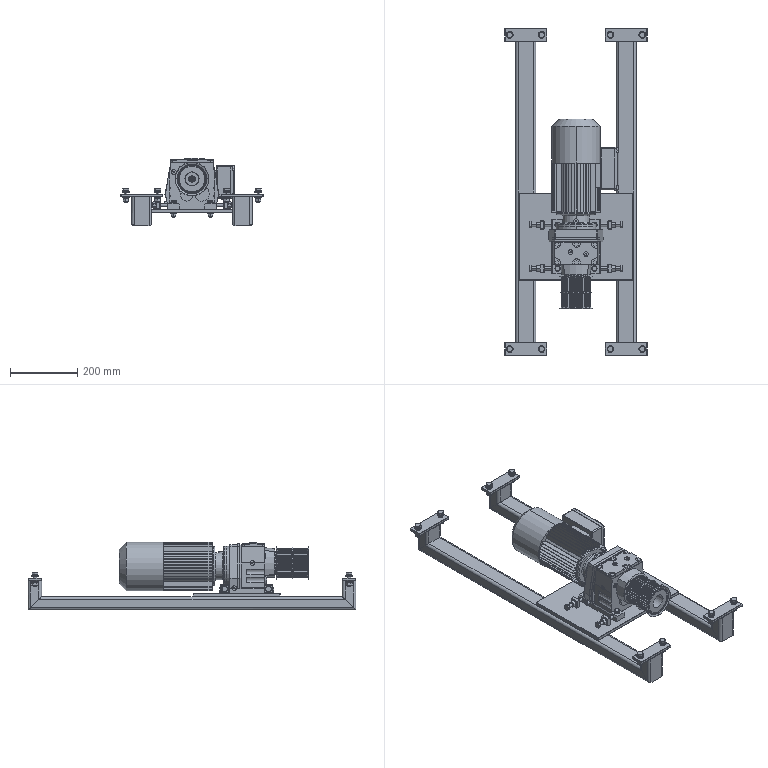Part | SolidWorks | 81 solids | 3091 faces | volume 10349735 mm3 | plane 1545 | cylinder 978 | cone 521 | spline 47 | commonest cylinder face diameters 1.6 x168 5.14 x168 85.208 x70 10 x60 8 x59 20 x43